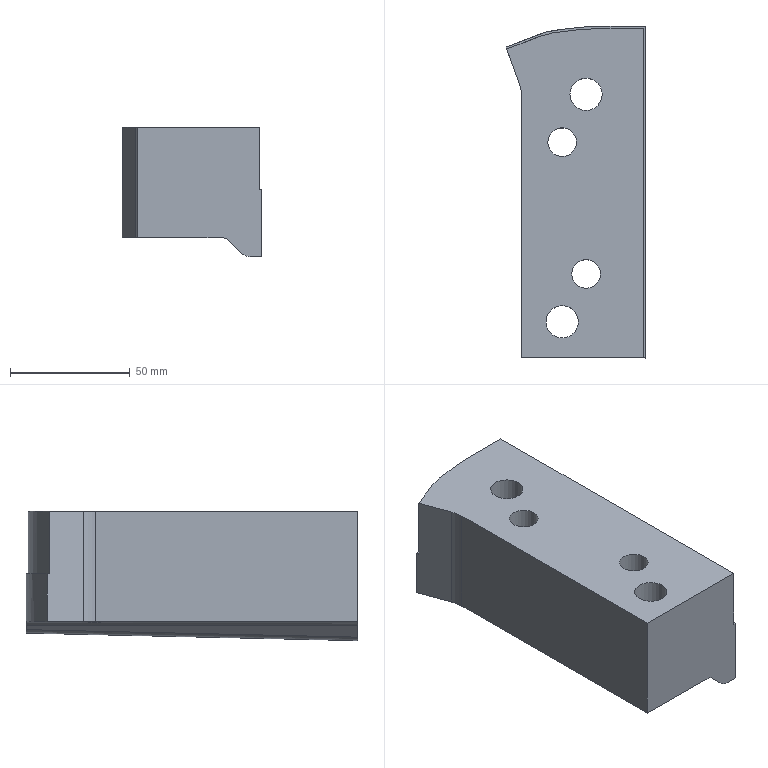Part | NX | features solid 2 | 1 solid | 27 faces | box 58.448 x 138.583 x 54 mm | volume 307683 mm3 | plane 14 | cylinder 11 | spline 2 | commonest cylinder face diameters 10 x2 12 x2 13 x2 13.5 x2 19.5 x2 30 x1
STEP:
#1=CARTESIAN_POINT('',(-128.106,-103.122,40.));
#2=VERTEX_POINT('',#1);
#3=CARTESIAN_POINT('',(-71.,-94.425,40.));
#4=VERTEX_POINT('',#3);
#5=CARTESIAN_POINT('',(-128.106,-103.122,40.));
#6=CARTESIAN_POINT('',(-125.791,-102.343,40.));
#7=CARTESIAN_POINT('',(-121.178,-100.674,40.));
#8=CARTESIAN_POINT('',(-115.494,-98.056,40.));
#9=CARTESIAN_POINT('',(-110.841,-96.645,40.));
#10=CARTESIAN_POINT('',(-107.28,-96.048,40.));
#11=CARTESIAN_POINT('',(-103.692,-95.631,40.));
#12=CARTESIAN_POINT('',(-98.907,-95.073,40.));
#13=CARTESIAN_POINT('',(-92.898,-94.557,40.));
#14=CARTESIAN_POINT('',(-85.612,-94.429,40.));
#15=CARTESIAN_POINT('',(-78.299,-94.474,40.));
#16=CARTESIAN_POINT('',(-73.433,-94.443,40.));
#17=CARTESIAN_POINT('',(-71.,-94.425,40.));
#18=B_SPLINE_CURVE_WITH_KNOTS('',3,(#5,#6,#7,#8,#9,#10,#11,#12,#13,#14,#15,#16,#17),.UNSPECIFIED.,.F.,.F.,(4,1,1,1,1,1,1,1,1,1,4),(0.0007141,0.007935,0.01516,0.01877,0.02238,0.02599,0.0296,0.03682,0.04404,0.05126,0.05848),.UNSPECIFIED.);
#19=EDGE_CURVE('',#2,#4,#18,.T.);
#20=ORIENTED_EDGE('',*,*,#19,.F.);
#21=CARTESIAN_POINT('',(-122.905,-117.413,40.));
#22=VERTEX_POINT('',#21);
#23=CARTESIAN_POINT('',(-206.143,111.282,40.));
#24=DIRECTION('',(0.342,-0.9397,0.));
#25=VECTOR('',#24,1000.);
#26=LINE('',#23,#25);
#27=EDGE_CURVE('',#2,#22,#26,.T.);
#28=ORIENTED_EDGE('',*,*,#27,.T.);
#29=CARTESIAN_POINT('',(-122.,-122.543,40.));
#30=VERTEX_POINT('',#29);
#31=CARTESIAN_POINT('',(-137.,-122.543,40.));
#32=DIRECTION('',(0.,0.,1.));
#33=DIRECTION('',(1.,0.,0.));
#34=AXIS2_PLACEMENT_3D('',#31,#32,#33);
#35=CIRCLE('',#34,15.);
#36=EDGE_CURVE('',#22,#30,#35,.F.);
#37=ORIENTED_EDGE('',*,*,#36,.T.);
#38=CARTESIAN_POINT('',(-122.,-232.,40.));
#39=VERTEX_POINT('',#38);
#40=CARTESIAN_POINT('',(-122.,35.09,40.));
#41=DIRECTION('',(0.,1.,0.));
#42=VECTOR('',#41,1000.);
#43=LINE('',#40,#42);
#44=EDGE_CURVE('',#39,#30,#43,.T.);
#45=ORIENTED_EDGE('',*,*,#44,.F.);
#46=CARTESIAN_POINT('',(-71.,-232.,40.));
#47=VERTEX_POINT('',#46);
#48=CARTESIAN_POINT('',(-415.478,-232.,40.));
#49=DIRECTION('',(1.,0.,0.));
#50=VECTOR('',#49,1000.);
#51=LINE('',#48,#50);
#52=EDGE_CURVE('',#47,#39,#51,.F.);
#53=ORIENTED_EDGE('',*,*,#52,.F.);
#54=CARTESIAN_POINT('',(-71.,35.09,40.));
#55=DIRECTION('',(0.,1.,0.));
#56=VECTOR('',#55,1000.);
#57=LINE('',#54,#56);
#58=EDGE_CURVE('',#47,#4,#57,.T.);
#59=ORIENTED_EDGE('',*,*,#58,.T.);
#60=EDGE_LOOP('',(#20,#28,#37,#45,#53,#59));
#61=FACE_BOUND('',#60,.T.);
#62=CARTESIAN_POINT('',(-89.,-197.,40.));
#63=VERTEX_POINT('',#62);
#64=CARTESIAN_POINT('',(-95.,-197.,40.));
#65=DIRECTION('',(0.,0.,1.));
#66=DIRECTION('',(1.,0.,0.));
#67=AXIS2_PLACEMENT_3D('',#64,#65,#66);
#68=CIRCLE('',#67,6.);
#69=EDGE_CURVE('',#63,#63,#68,.T.);
#70=ORIENTED_EDGE('',*,*,#69,.F.);
#71=EDGE_LOOP('',(#70));
#72=FACE_BOUND('',#71,.T.);
#73=CARTESIAN_POINT('',(-99.,-142.,40.));
#74=VERTEX_POINT('',#73);
#75=CARTESIAN_POINT('',(-105.,-142.,40.));
#76=DIRECTION('',(0.,0.,1.));
#77=DIRECTION('',(1.,0.,0.));
#78=AXIS2_PLACEMENT_3D('',#75,#76,#77);
#79=CIRCLE('',#78,6.);
#80=EDGE_CURVE('',#74,#74,#79,.T.);
#81=ORIENTED_EDGE('',*,*,#80,.F.);
#82=EDGE_LOOP('',(#81));
#83=FACE_BOUND('',#82,.T.);
#84=CARTESIAN_POINT('',(-88.25,-122.,40.));
#85=VERTEX_POINT('',#84);
#86=CARTESIAN_POINT('',(-95.,-122.,40.));
#87=DIRECTION('',(0.,0.,1.));
#88=DIRECTION('',(1.,0.,0.));
#89=AXIS2_PLACEMENT_3D('',#86,#87,#88);
#90=CIRCLE('',#89,6.75);
#91=EDGE_CURVE('',#85,#85,#90,.T.);
#92=ORIENTED_EDGE('',*,*,#91,.F.);
#93=EDGE_LOOP('',(#92));
#94=FACE_BOUND('',#93,.T.);
#95=CARTESIAN_POINT('',(-98.25,-217.,40.));
#96=VERTEX_POINT('',#95);
#97=CARTESIAN_POINT('',(-105.,-217.,40.));
#98=DIRECTION('',(0.,0.,1.));
#99=DIRECTION('',(1.,0.,0.));
#100=AXIS2_PLACEMENT_3D('',#97,#98,#99);
#101=CIRCLE('',#100,6.75);
#102=EDGE_CURVE('',#96,#96,#101,.T.);
#103=ORIENTED_EDGE('',*,*,#102,.F.);
#104=EDGE_LOOP('',(#103));
#105=FACE_BOUND('',#104,.T.);
#106=CARTESIAN_POINT('',(-415.478,35.09,40.));
#107=DIRECTION('',(0.,0.,1.));
#108=DIRECTION('',(1.,0.,0.));
#109=AXIS2_PLACEMENT_3D('',#106,#107,#108);
#110=PLANE('',#109);
#111=ADVANCED_FACE('',(#61,#72,#83,#94,#105),#110,.T.);
#112=CARTESIAN_POINT('',(-70.,-93.417,14.));
#113=VERTEX_POINT('',#112);
#114=CARTESIAN_POINT('',(-70.,-232.,14.));
#115=VERTEX_POINT('',#114);
#116=CARTESIAN_POINT('',(-70.,-99.381,14.));
#117=DIRECTION('',(0.,-1.,0.));
#118=VECTOR('',#117,1000.);
#119=LINE('',#116,#118);
#120=EDGE_CURVE('',#113,#115,#119,.T.);
#121=ORIENTED_EDGE('',*,*,#120,.T.);
#122=CARTESIAN_POINT('',(-70.,-232.,-14.));
#123=VERTEX_POINT('',#122);
#124=CARTESIAN_POINT('',(-70.,-232.,-66.));
#125=DIRECTION('',(0.,0.,1.));
#126=VECTOR('',#125,1000.);
#127=LINE('',#124,#126);
#128=EDGE_CURVE('',#115,#123,#127,.F.);
#129=ORIENTED_EDGE('',*,*,#128,.T.);
#130=CARTESIAN_POINT('',(-70.,-93.417,-10.865));
#131=VERTEX_POINT('',#130);
#132=CARTESIAN_POINT('',(-70.,-231.932,-13.998));
#133=DIRECTION('',(0.,0.9997,0.02262));
#134=VECTOR('',#133,1000.);
#135=LINE('',#132,#134);
#136=EDGE_CURVE('',#123,#131,#135,.T.);
#137=ORIENTED_EDGE('',*,*,#136,.T.);
#138=CARTESIAN_POINT('',(-70.,-93.417,1.5));
#139=DIRECTION('',(0.,0.,-1.));
#140=VECTOR('',#139,1000.);
#141=LINE('',#138,#140);
#142=EDGE_CURVE('',#131,#113,#141,.F.);
#143=ORIENTED_EDGE('',*,*,#142,.T.);
#144=EDGE_LOOP('',(#121,#129,#137,#143));
#145=FACE_BOUND('',#144,.T.);
#146=CARTESIAN_POINT('',(-70.,-99.381,-66.));
#147=DIRECTION('',(-1.,0.,0.));
#148=DIRECTION('',(0.,0.,1.));
#149=AXIS2_PLACEMENT_3D('',#146,#147,#148);
#150=PLANE('',#149);
#151=ADVANCED_FACE('',(#145),#150,.F.);
#152=CARTESIAN_POINT('',(-83.536,-232.,-7.464));
#153=VERTEX_POINT('',#152);
#154=CARTESIAN_POINT('',(-78.467,-232.,-12.533));
#155=VERTEX_POINT('',#154);
#156=CARTESIAN_POINT('',(-42.,-232.,-49.));
#157=DIRECTION('',(0.7071,0.,-0.7071));
#158=VECTOR('',#157,1000.);
#159=LINE('',#156,#158);
#160=EDGE_CURVE('',#153,#155,#159,.T.);
#161=ORIENTED_EDGE('',*,*,#160,.T.);
#162=CARTESIAN_POINT('',(-74.929,-232.,-13.999));
#163=VERTEX_POINT('',#162);
#164=CARTESIAN_POINT('',(-74.931,-232.,-8.998));
#165=DIRECTION('',(0.,-1.,0.));
#166=DIRECTION('',(0.7071,0.,-0.7071));
#167=AXIS2_PLACEMENT_3D('',#164,#165,#166);
#168=ELLIPSE('',#167,5.003,5.);
#169=EDGE_CURVE('',#155,#163,#168,.T.);
#170=ORIENTED_EDGE('',*,*,#169,.T.);
#171=CARTESIAN_POINT('',(-90.001,-232.,-13.996));
#172=DIRECTION('',(1.,0.,-0.0001826));
#173=VECTOR('',#172,1000.);
#174=LINE('',#171,#173);
#175=EDGE_CURVE('',#163,#123,#174,.T.);
#176=ORIENTED_EDGE('',*,*,#175,.T.);
#177=ORIENTED_EDGE('',*,*,#128,.F.);
#178=CARTESIAN_POINT('',(-71.,-232.,14.));
#179=VERTEX_POINT('',#178);
#180=CARTESIAN_POINT('',(-454.349,-232.,14.));
#181=DIRECTION('',(-1.,0.,0.));
#182=VECTOR('',#181,1000.);
#183=LINE('',#180,#182);
#184=EDGE_CURVE('',#179,#115,#183,.F.);
#185=ORIENTED_EDGE('',*,*,#184,.F.);
#186=CARTESIAN_POINT('',(-71.,-232.,14.));
#187=DIRECTION('',(0.,0.,-1.));
#188=VECTOR('',#187,1000.);
#189=LINE('',#186,#188);
#190=EDGE_CURVE('',#179,#47,#189,.F.);
#191=ORIENTED_EDGE('',*,*,#190,.T.);
#192=ORIENTED_EDGE('',*,*,#52,.T.);
#193=CARTESIAN_POINT('',(-122.,-232.,-6.));
#194=VERTEX_POINT('',#193);
#195=CARTESIAN_POINT('',(-122.,-232.,-67.));
#196=DIRECTION('',(0.,0.,1.));
#197=VECTOR('',#196,1000.);
#198=LINE('',#195,#197);
#199=EDGE_CURVE('',#39,#194,#198,.F.);
#200=ORIENTED_EDGE('',*,*,#199,.T.);
#201=CARTESIAN_POINT('',(-87.071,-232.,-6.));
#202=VERTEX_POINT('',#201);
#203=CARTESIAN_POINT('',(-470.381,-232.,-6.));
#204=DIRECTION('',(-1.,0.,0.));
#205=VECTOR('',#204,1000.);
#206=LINE('',#203,#205);
#207=EDGE_CURVE('',#194,#202,#206,.F.);
#208=ORIENTED_EDGE('',*,*,#207,.T.);
#209=CARTESIAN_POINT('',(-87.071,-232.,-11.));
#210=DIRECTION('',(0.,-1.,0.));
#211=DIRECTION('',(0.,0.,-1.));
#212=AXIS2_PLACEMENT_3D('',#209,#210,#211);
#213=CIRCLE('',#212,5.);
#214=EDGE_CURVE('',#202,#153,#213,.F.);
#215=ORIENTED_EDGE('',*,*,#214,.T.);
#216=EDGE_LOOP('',(#161,#170,#176,#177,#185,#191,#192,#200,#208,#215));
#217=FACE_BOUND('',#216,.T.);
#218=CARTESIAN_POINT('',(-70.,-232.,-67.));
#219=DIRECTION('',(0.,-1.,0.));
#220=DIRECTION('',(0.,0.,1.));
#221=AXIS2_PLACEMENT_3D('',#218,#219,#220);
#222=PLANE('',#221);
#223=ADVANCED_FACE('',(#217),#222,.T.);
#224=CARTESIAN_POINT('',(-88.5,-197.,-6.));
#225=VERTEX_POINT('',#224);
#226=CARTESIAN_POINT('',(-95.,-197.,-6.));
#227=DIRECTION('',(0.,0.,1.));
#228=DIRECTION('',(1.,0.,0.));
#229=AXIS2_PLACEMENT_3D('',#226,#227,#228);
#230=CIRCLE('',#229,6.5);
#231=EDGE_CURVE('',#225,#225,#230,.T.);
#232=ORIENTED_EDGE('',*,*,#231,.T.);
#233=EDGE_LOOP('',(#232));
#234=FACE_BOUND('',#233,.T.);
#235=CARTESIAN_POINT('',(-98.5,-142.,-6.));
#236=VERTEX_POINT('',#235);
#237=CARTESIAN_POINT('',(-105.,-142.,-6.));
#238=DIRECTION('',(0.,0.,1.));
#239=DIRECTION('',(1.,0.,0.));
#240=AXIS2_PLACEMENT_3D('',#237,#238,#239);
#241=CIRCLE('',#240,6.5);
#242=EDGE_CURVE('',#236,#236,#241,.T.);
#243=ORIENTED_EDGE('',*,*,#242,.T.);
#244=EDGE_LOOP('',(#243));
#245=FACE_BOUND('',#244,.T.);
#246=CARTESIAN_POINT('',(-128.448,-102.182,-6.));
#247=VERTEX_POINT('',#246);
#248=CARTESIAN_POINT('',(-87.071,-93.469,-6.));
#249=VERTEX_POINT('',#248);
#250=CARTESIAN_POINT('',(-128.448,-102.182,-6.));
#251=CARTESIAN_POINT('',(-126.732,-101.605,-6.));
#252=CARTESIAN_POINT('',(-123.317,-100.412,-6.));
#253=CARTESIAN_POINT('',(-118.327,-98.259,-6.));
#254=CARTESIAN_POINT('',(-113.316,-96.192,-6.));
#255=CARTESIAN_POINT('',(-108.153,-95.109,-6.));
#256=CARTESIAN_POINT('',(-102.907,-94.545,-6.));
#257=CARTESIAN_POINT('',(-97.669,-93.925,-6.));
#258=CARTESIAN_POINT('',(-92.389,-93.579,-6.));
#259=CARTESIAN_POINT('',(-88.846,-93.489,-6.));
#260=CARTESIAN_POINT('',(-87.071,-93.469,-6.));
#261=B_SPLINE_CURVE_WITH_KNOTS('',3,(#250,#251,#252,#253,#254,#255,#256,#257,#258,#259,#260),.UNSPECIFIED.,.F.,.F.,(4,1,1,1,1,1,1,1,4),(-0.008773,-0.003503,0.001767,0.007037,0.01231,0.01758,0.02285,0.02812,0.03339),.UNSPECIFIED.);
#262=EDGE_CURVE('',#247,#249,#261,.T.);
#263=ORIENTED_EDGE('',*,*,#262,.T.);
#264=CARTESIAN_POINT('',(-87.071,-116.326,-6.));
#265=VERTEX_POINT('',#264);
#266=CARTESIAN_POINT('',(-87.071,-222.,-6.));
#267=DIRECTION('',(0.,1.,0.));
#268=VECTOR('',#267,1000.);
#269=LINE('',#266,#268);
#270=EDGE_CURVE('',#249,#265,#269,.F.);
#271=ORIENTED_EDGE('',*,*,#270,.T.);
#272=CARTESIAN_POINT('',(-87.071,-127.674,-6.));
#273=VERTEX_POINT('',#272);
#274=CARTESIAN_POINT('',(-95.,-122.,-6.));
#275=DIRECTION('',(0.,0.,1.));
#276=DIRECTION('',(1.,0.,0.));
#277=AXIS2_PLACEMENT_3D('',#274,#275,#276);
#278=CIRCLE('',#277,9.75);
#279=EDGE_CURVE('',#265,#273,#278,.T.);
#280=ORIENTED_EDGE('',*,*,#279,.T.);
#281=CARTESIAN_POINT('',(-87.071,-222.,-6.));
#282=DIRECTION('',(0.,1.,0.));
#283=VECTOR('',#282,1000.);
#284=LINE('',#281,#283);
#285=EDGE_CURVE('',#273,#202,#284,.F.);
#286=ORIENTED_EDGE('',*,*,#285,.T.);
#287=ORIENTED_EDGE('',*,*,#207,.F.);
#288=CARTESIAN_POINT('',(-122.,-122.543,-6.));
#289=VERTEX_POINT('',#288);
#290=CARTESIAN_POINT('',(-122.,-222.,-6.));
#291=DIRECTION('',(0.,-1.,0.));
#292=VECTOR('',#291,1000.);
#293=LINE('',#290,#292);
#294=EDGE_CURVE('',#289,#194,#293,.T.);
#295=ORIENTED_EDGE('',*,*,#294,.F.);
#296=CARTESIAN_POINT('',(-122.905,-117.413,-6.));
#297=VERTEX_POINT('',#296);
#298=CARTESIAN_POINT('',(-137.,-122.543,-6.));
#299=DIRECTION('',(0.,0.,-1.));
#300=DIRECTION('',(-1.,0.,0.));
#301=AXIS2_PLACEMENT_3D('',#298,#299,#300);
#302=CIRCLE('',#301,15.);
#303=EDGE_CURVE('',#289,#297,#302,.F.);
#304=ORIENTED_EDGE('',*,*,#303,.T.);
#305=CARTESIAN_POINT('',(-129.938,-98.089,-6.));
#306=DIRECTION('',(-0.342,0.9397,0.));
#307=VECTOR('',#306,1000.);
#308=LINE('',#305,#307);
#309=EDGE_CURVE('',#297,#247,#308,.T.);
#310=ORIENTED_EDGE('',*,*,#309,.T.);
#311=EDGE_LOOP('',(#263,#271,#280,#286,#287,#295,#304,#310));
#312=FACE_BOUND('',#311,.T.);
#313=CARTESIAN_POINT('',(-95.25,-217.,-6.));
#314=VERTEX_POINT('',#313);
#315=CARTESIAN_POINT('',(-105.,-217.,-6.));
#316=DIRECTION('',(0.,0.,1.));
#317=DIRECTION('',(1.,0.,0.));
#318=AXIS2_PLACEMENT_3D('',#315,#316,#317);
#319=CIRCLE('',#318,9.75);
#320=EDGE_CURVE('',#314,#314,#319,.T.);
#321=ORIENTED_EDGE('',*,*,#320,.T.);
#322=EDGE_LOOP('',(#321));
#323=FACE_BOUND('',#322,.T.);
#324=CARTESIAN_POINT('',(-470.381,-222.,-6.));
#325=DIRECTION('',(0.,0.,-1.));
#326=DIRECTION('',(-1.,0.,0.));
#327=AXIS2_PLACEMENT_3D('',#324,#325,#326);
#328=PLANE('',#327);
#329=ADVANCED_FACE('',(#234,#245,#312,#323),#328,.T.);
#330=CARTESIAN_POINT('',(-78.064,-93.458,-10.865));
#331=VERTEX_POINT('',#330);
#332=CARTESIAN_POINT('',(-78.064,-93.458,-10.865));
#333=CARTESIAN_POINT('',(-75.376,-93.455,-10.865));
#334=CARTESIAN_POINT('',(-72.688,-93.438,-10.865));
#335=CARTESIAN_POINT('',(-70.,-93.417,-10.865));
#336=B_SPLINE_CURVE_WITH_KNOTS('',3,(#332,#333,#334,#335),.UNSPECIFIED.,.F.,.F.,(4,4),(0.002072,0.01014),.UNSPECIFIED.);
#337=EDGE_CURVE('',#331,#131,#336,.T.);
#338=ORIENTED_EDGE('',*,*,#337,.F.);
#339=CARTESIAN_POINT('',(-81.601,-93.455,-9.399));
#340=VERTEX_POINT('',#339);
#341=CARTESIAN_POINT('',(-78.064,-93.458,-10.865));
#342=CARTESIAN_POINT('',(-79.385,-93.46,-10.864));
#343=CARTESIAN_POINT('',(-80.667,-93.457,-10.333));
#344=CARTESIAN_POINT('',(-81.601,-93.455,-9.399));
#345=B_SPLINE_CURVE_WITH_KNOTS('',3,(#341,#342,#343,#344),.UNSPECIFIED.,.F.,.F.,(4,4),(0.,0.003906),.UNSPECIFIED.);
#346=EDGE_CURVE('',#331,#340,#345,.T.);
#347=ORIENTED_EDGE('',*,*,#346,.T.);
#348=CARTESIAN_POINT('',(-83.536,-93.453,-7.464));
#349=VERTEX_POINT('',#348);
#350=CARTESIAN_POINT('',(-81.601,-93.455,-9.399));
#351=CARTESIAN_POINT('',(-82.246,-93.454,-8.754));
#352=CARTESIAN_POINT('',(-82.891,-93.453,-8.109));
#353=CARTESIAN_POINT('',(-83.536,-93.453,-7.464));
#354=B_SPLINE_CURVE_WITH_KNOTS('',3,(#350,#351,#352,#353),.UNSPECIFIED.,.F.,.F.,(4,4),(0.002072,0.004808),.UNSPECIFIED.);
#355=EDGE_CURVE('',#340,#349,#354,.T.);
#356=ORIENTED_EDGE('',*,*,#355,.T.);
#357=CARTESIAN_POINT('',(-83.536,-93.453,-7.464));
#358=CARTESIAN_POINT('',(-84.469,-93.453,-6.531));
#359=CARTESIAN_POINT('',(-85.751,-93.455,-6.));
#360=CARTESIAN_POINT('',(-87.071,-93.469,-6.));
#361=B_SPLINE_CURVE_WITH_KNOTS('',3,(#357,#358,#359,#360),.UNSPECIFIED.,.F.,.F.,(4,4),(0.,0.003904),.UNSPECIFIED.);
#362=EDGE_CURVE('',#349,#249,#361,.T.);
#363=ORIENTED_EDGE('',*,*,#362,.T.);
#364=ORIENTED_EDGE('',*,*,#262,.F.);
#365=CARTESIAN_POINT('',(-128.448,-102.182,14.));
#366=VERTEX_POINT('',#365);
#367=CARTESIAN_POINT('',(-128.448,-102.182,15.35));
#368=DIRECTION('',(0.,0.,-1.));
#369=VECTOR('',#368,1000.);
#370=LINE('',#367,#369);
#371=EDGE_CURVE('',#247,#366,#370,.F.);
#372=ORIENTED_EDGE('',*,*,#371,.T.);
#373=CARTESIAN_POINT('',(-71.,-93.425,14.));
#374=VERTEX_POINT('',#373);
#375=CARTESIAN_POINT('',(-190.231,-121.49,14.));
#376=CARTESIAN_POINT('',(-188.654,-121.152,14.));
#377=CARTESIAN_POINT('',(-185.47,-120.627,14.));
#378=CARTESIAN_POINT('',(-180.656,-120.141,14.));
#379=CARTESIAN_POINT('',(-175.882,-119.326,14.));
#380=CARTESIAN_POINT('',(-169.679,-117.528,14.));
#381=CARTESIAN_POINT('',(-162.185,-114.539,14.));
#382=CARTESIAN_POINT('',(-153.086,-111.254,14.));
#383=CARTESIAN_POINT('',(-144.031,-107.845,14.));
#384=CARTESIAN_POINT('',(-136.465,-105.061,14.));
#385=CARTESIAN_POINT('',(-130.418,-102.814,14.));
#386=CARTESIAN_POINT('',(-125.812,-101.329,14.));
#387=CARTESIAN_POINT('',(-121.306,-99.566,14.));
#388=CARTESIAN_POINT('',(-116.876,-97.626,14.));
#389=CARTESIAN_POINT('',(-112.335,-95.923,14.));
#390=CARTESIAN_POINT('',(-107.564,-95.05,14.));
#391=CARTESIAN_POINT('',(-102.756,-94.525,14.));
#392=CARTESIAN_POINT('',(-96.349,-93.771,14.));
#393=CARTESIAN_POINT('',(-89.902,-93.468,14.));
#394=CARTESIAN_POINT('',(-83.452,-93.448,14.));
#395=CARTESIAN_POINT('',(-77.002,-93.469,14.));
#396=CARTESIAN_POINT('',(-68.939,-93.411,14.));
#397=CARTESIAN_POINT('',(-56.04,-93.3,14.));
#398=CARTESIAN_POINT('',(-33.465,-93.184,14.));
#399=CARTESIAN_POINT('',(-7.666,-93.074,14.));
#400=CARTESIAN_POINT('',(14.907,-92.653,14.));
#401=CARTESIAN_POINT('',(27.794,-92.068,14.));
#402=CARTESIAN_POINT('',(40.668,-91.245,14.));
#403=CARTESIAN_POINT('',(51.917,-90.291,14.));
#404=CARTESIAN_POINT('',(61.528,-89.174,14.));
#405=CARTESIAN_POINT('',(67.939,-88.466,14.));
#406=CARTESIAN_POINT('',(79.125,-86.95,14.));
#407=CARTESIAN_POINT('',(95.161,-85.253,14.));
#408=CARTESIAN_POINT('',(114.404,-83.21,14.));
#409=CARTESIAN_POINT('',(133.568,-80.524,14.));
#410=CARTESIAN_POINT('',(152.734,-77.861,14.));
#411=CARTESIAN_POINT('',(171.916,-75.326,14.));
#412=CARTESIAN_POINT('',(191.055,-72.413,14.));
#413=CARTESIAN_POINT('',(207.17,-71.468,14.));
#414=CARTESIAN_POINT('',(219.951,-69.697,14.));
#415=CARTESIAN_POINT('',(232.724,-67.899,14.));
#416=CARTESIAN_POINT('',(248.708,-65.766,14.));
#417=CARTESIAN_POINT('',(267.87,-63.074,14.));
#418=CARTESIAN_POINT('',(287.038,-60.44,14.));
#419=CARTESIAN_POINT('',(301.448,-58.682,14.));
#420=CARTESIAN_POINT('',(310.976,-56.987,14.));
#421=CARTESIAN_POINT('',(314.916,-56.135,14.));
#422=CARTESIAN_POINT('',(318.052,-55.382,14.));
#423=CARTESIAN_POINT('',(320.39,-54.76,14.));
#424=CARTESIAN_POINT('',(322.686,-53.981,14.));
#425=CARTESIAN_POINT('',(325.595,-52.578,14.));
#426=CARTESIAN_POINT('',(328.769,-50.098,14.));
#427=CARTESIAN_POINT('',(332.247,-46.69,14.));
#428=CARTESIAN_POINT('',(335.795,-43.406,14.));
#429=CARTESIAN_POINT('',(343.661,-37.758,14.));
#430=CARTESIAN_POINT('',(355.164,-28.914,14.));
#431=CARTESIAN_POINT('',(370.422,-17.018,14.));
#432=CARTESIAN_POINT('',(383.264,-7.249,14.));
#433=CARTESIAN_POINT('',(392.416,-0.6713,14.));
#434=CARTESIAN_POINT('',(396.953,2.733,14.));
#435=CARTESIAN_POINT('',(398.886,5.372,14.));
#436=CARTESIAN_POINT('',(399.725,7.654,14.));
#437=CARTESIAN_POINT('',(399.76,10.078,14.));
#438=CARTESIAN_POINT('',(399.483,13.317,14.));
#439=CARTESIAN_POINT('',(399.712,17.34,14.));
#440=CARTESIAN_POINT('',(399.612,22.179,14.));
#441=CARTESIAN_POINT('',(399.633,31.854,14.));
#442=CARTESIAN_POINT('',(399.593,46.366,14.));
#443=CARTESIAN_POINT('',(399.637,62.491,14.));
#444=CARTESIAN_POINT('',(399.588,73.779,14.));
#445=CARTESIAN_POINT('',(399.652,79.422,14.));
#446=CARTESIAN_POINT('',(399.59,82.647,14.));
#447=CARTESIAN_POINT('',(399.564,85.065,14.));
#448=CARTESIAN_POINT('',(399.725,87.486,14.));
#449=CARTESIAN_POINT('',(399.756,89.902,14.));
#450=CARTESIAN_POINT('',(399.247,92.301,14.));
#451=CARTESIAN_POINT('',(397.362,95.008,14.));
#452=CARTESIAN_POINT('',(393.635,96.774,14.));
#453=CARTESIAN_POINT('',(389.279,98.826,14.));
#454=CARTESIAN_POINT('',(384.732,100.498,14.));
#455=CARTESIAN_POINT('',(378.765,102.95,14.));
#456=CARTESIAN_POINT('',(362.589,110.229,14.));
#457=CARTESIAN_POINT('',(344.928,118.135,14.));
#458=CARTESIAN_POINT('',(327.281,126.072,14.));
#459=CARTESIAN_POINT('',(319.932,129.381,14.));
#460=CARTESIAN_POINT('',(314.075,132.102,14.));
#461=CARTESIAN_POINT('',(309.387,133.376,14.));
#462=CARTESIAN_POINT('',(304.547,133.785,14.));
#463=CARTESIAN_POINT('',(299.716,133.401,14.));
#464=CARTESIAN_POINT('',(294.929,132.704,14.));
#465=CARTESIAN_POINT('',(288.543,131.8,14.));
#466=CARTESIAN_POINT('',(277.364,130.241,14.));
#467=CARTESIAN_POINT('',(242.2,125.552,14.));
#468=CARTESIAN_POINT('',(184.637,118.048,14.));
#469=CARTESIAN_POINT('',(120.701,109.541,14.));
#470=CARTESIAN_POINT('',(69.531,102.902,14.));
#471=CARTESIAN_POINT('',(40.777,98.94,14.));
#472=CARTESIAN_POINT('',(21.566,96.615,14.));
#473=CARTESIAN_POINT('',(8.743,95.212,14.));
#474=CARTESIAN_POINT('',(-7.301,93.575,14.));
#475=CARTESIAN_POINT('',(-26.625,92.505,14.));
#476=CARTESIAN_POINT('',(-45.971,92.017,14.));
#477=CARTESIAN_POINT('',(-62.09,91.675,14.));
#478=CARTESIAN_POINT('',(-74.987,91.256,14.));
#479=CARTESIAN_POINT('',(-84.664,91.165,14.));
#480=CARTESIAN_POINT('',(-94.319,91.781,14.));
#481=CARTESIAN_POINT('',(-103.929,92.966,14.));
#482=CARTESIAN_POINT('',(-113.495,94.403,14.));
#483=CARTESIAN_POINT('',(-119.856,95.492,14.));
#484=CARTESIAN_POINT('',(-122.997,96.222,14.));
#485=B_SPLINE_CURVE_WITH_KNOTS('',3,(#375,#376,#377,#378,#379,#380,#381,#382,#383,#384,#385,#386,#387,#388,#389,#390,#391,#392,#393,#394,#395,#396,#397,#398,#399,#400,#401,#402,#403,#404,#405,#406,#407,#408,#409,#410,#411,#412,#413,#414,#415,#416,#417,#418,#419,#420,#421,#422,#423,#424,#425,#426,#427,#428,#429,#430,#431,#432,#433,#434,#435,#436,#437,#438,#439,#440,#441,#442,#443,#444,#445,#446,#447,#448,#449,#450,#451,#452,#453,#454,#455,#456,#457,#458,#459,#460,#461,#462,#463,#464,#465,#466,#467,#468,#469,#470,#471,#472,#473,#474,#475,#476,#477,#478,#479,#480,#481,#482,#483,#484),.UNSPECIFIED.,.F.,.F.,(4,1,1,1,1,1,1,1,1,1,1,1,1,1,1,1,1,1,1,1,1,1,1,1,1,1,1,1,1,1,1,1,1,1,1,1,1,1,1,1,1,1,1,1,1,1,1,1,1,1,1,1,1,1,1,1,1,1,1,1,1,1,1,1,1,1,1,1,1,1,1,1,1,1,1,1,1,1,1,1,1,1,1,1,1,1,1,1,1,1,1,1,1,1,1,1,1,1,1,1,1,1,1,1,1,1,1,4),(0.4704,0.4724,0.4745,0.4766,0.4786,0.4828,0.4869,0.491,0.4952,0.4972,0.4993,0.5014,0.5035,0.5055,0.5076,0.5097,0.5117,0.5159,0.5179,0.52,0.5241,0.5283,0.5366,0.5531,0.5614,0.5655,0.5697,0.5779,0.58,0.5821,0.5862,0.5945,0.6028,0.611,0.6193,0.6276,0.6359,0.6441,0.6483,0.6524,0.6607,0.669,0.6772,0.6855,0.6876,0.6897,0.6907,0.6917,0.6928,0.6938,0.6959,0.6979,0.7,0.7021,0.7103,0.7186,0.7269,0.731,0.7331,0.7341,0.7352,0.7362,0.7372,0.7393,0.7414,0.7435,0.7517,0.76,0.7641,0.7662,0.7672,0.7683,0.7693,0.7703,0.7714,0.7724,0.7745,0.7766,0.7786,0.7807,0.7848,0.8014,0.8055,0.8097,0.8117,0.8138,0.8159,0.8179,0.82,0.8221,0.8262,0.8345,0.8676,0.9007,0.9172,0.9338,0.9379,0.9421,0.9503,0.9586,0.9669,0.9752,0.9793,0.9834,0.9876,0.9917,0.9959,1.),.UNSPECIFIED.);
#486=EDGE_CURVE('',#374,#366,#485,.F.);
#487=ORIENTED_EDGE('',*,*,#486,.F.);
#488=CARTESIAN_POINT('',(-70.,-93.417,14.));
#489=CARTESIAN_POINT('',(-70.333,-93.42,14.));
#490=CARTESIAN_POINT('',(-70.667,-93.422,14.));
#491=CARTESIAN_POINT('',(-71.,-93.425,14.));
#492=B_SPLINE_CURVE_WITH_KNOTS('',3,(#488,#489,#490,#491),.UNSPECIFIED.,.F.,.F.,(4,4),(0.,0.0009947),.UNSPECIFIED.);
#493=EDGE_CURVE('',#113,#374,#492,.T.);
#494=ORIENTED_EDGE('',*,*,#493,.F.);
#495=ORIENTED_EDGE('',*,*,#142,.F.);
#496=EDGE_LOOP('',(#338,#347,#356,#363,#364,#372,#487,#494,#495));
#497=FACE_BOUND('',#496,.T.);
#498=CARTESIAN_POINT('',(-128.448,-102.182,14.));
#499=CARTESIAN_POINT('',(-128.448,-102.182,-11.014));
#500=CARTESIAN_POINT('',(-126.088,-101.388,14.));
#501=CARTESIAN_POINT('',(-126.088,-101.388,-11.014));
#502=CARTESIAN_POINT('',(-121.41,-99.687,14.));
#503=CARTESIAN_POINT('',(-121.41,-99.687,-11.014));
#504=CARTESIAN_POINT('',(-115.74,-97.072,14.));
#505=CARTESIAN_POINT('',(-115.74,-97.072,-11.014));
#506=CARTESIAN_POINT('',(-110.967,-95.647,14.));
#507=CARTESIAN_POINT('',(-110.967,-95.647,-11.014));
#508=CARTESIAN_POINT('',(-107.273,-95.036,14.));
#509=CARTESIAN_POINT('',(-107.273,-95.036,-11.014));
#510=CARTESIAN_POINT('',(-103.564,-94.612,14.));
#511=CARTESIAN_POINT('',(-103.564,-94.612,-11.014));
#512=CARTESIAN_POINT('',(-98.617,-94.031,14.));
#513=CARTESIAN_POINT('',(-98.617,-94.031,-11.014));
#514=CARTESIAN_POINT('',(-92.411,-93.532,14.));
#515=CARTESIAN_POINT('',(-92.411,-93.532,-11.014));
#516=CARTESIAN_POINT('',(-84.939,-93.431,14.));
#517=CARTESIAN_POINT('',(-84.939,-93.431,-11.014));
#518=CARTESIAN_POINT('',(-77.47,-93.474,14.));
#519=CARTESIAN_POINT('',(-77.47,-93.474,-11.014));
#520=CARTESIAN_POINT('',(-72.49,-93.436,14.));
#521=CARTESIAN_POINT('',(-72.49,-93.436,-11.014));
#522=CARTESIAN_POINT('',(-70.,-93.417,14.));
#523=CARTESIAN_POINT('',(-70.,-93.417,-11.014));
#524=B_SPLINE_SURFACE_WITH_KNOTS('',3,1,((#498,#499),(#500,#501),(#502,#503),(#504,#505),(#506,#507),(#508,#509),(#510,#511),(#512,#513),(#514,#515),(#516,#517),(#518,#519),(#520,#521),(#522,#523)),.SURF_OF_LINEAR_EXTRUSION.,.F.,.F.,.F.,(4,1,1,1,1,1,1,1,1,1,4),(2,2),(0.4981,0.5013,0.5045,0.5061,0.5077,0.5093,0.5109,0.5141,0.5173,0.5205,0.5237),(0.,1.),.UNSPECIFIED.);
#525=ADVANCED_FACE('',(#497),#524,.T.);
#526=ORIENTED_EDGE('',*,*,#44,.T.);
#527=CARTESIAN_POINT('',(-122.,-122.543,23.));
#528=DIRECTION('',(0.,0.,-1.));
#529=VECTOR('',#528,1000.);
#530=LINE('',#527,#529);
#531=EDGE_CURVE('',#30,#289,#530,.T.);
#532=ORIENTED_EDGE('',*,*,#531,.T.);
#533=ORIENTED_EDGE('',*,*,#294,.T.);
#534=ORIENTED_EDGE('',*,*,#199,.F.);
#535=EDGE_LOOP('',(#526,#532,#533,#534));
#536=FACE_BOUND('',#535,.T.);
#537=CARTESIAN_POINT('',(-122.,-169.69,23.));
#538=DIRECTION('',(1.,0.,0.));
#539=DIRECTION('',(0.,0.,-1.));
#540=AXIS2_PLACEMENT_3D('',#537,#538,#539);
#541=PLANE('',#540);
#542=ADVANCED_FACE('',(#536),#541,.F.);
#543=ORIENTED_EDGE('',*,*,#184,.T.);
#544=ORIENTED_EDGE('',*,*,#120,.F.);
#545=ORIENTED_EDGE('',*,*,#493,.T.);
#546=ORIENTED_EDGE('',*,*,#486,.T.);
#547=CARTESIAN_POINT('',(-128.106,-103.122,14.));
#548=VERTEX_POINT('',#547);
#549=CARTESIAN_POINT('',(-129.506,-99.275,14.));
#550=DIRECTION('',(0.342,-0.9397,0.));
#551=VECTOR('',#550,1000.);
#552=LINE('',#549,#551);
#553=EDGE_CURVE('',#366,#548,#552,.T.);
#554=ORIENTED_EDGE('',*,*,#553,.T.);
#555=CARTESIAN_POINT('',(-71.,-94.425,14.));
#556=VERTEX_POINT('',#555);
#557=CARTESIAN_POINT('',(-128.106,-103.122,14.));
#558=CARTESIAN_POINT('',(-125.786,-102.341,14.));
#559=CARTESIAN_POINT('',(-121.105,-100.639,14.));
#560=CARTESIAN_POINT('',(-115.535,-98.084,14.));
#561=CARTESIAN_POINT('',(-111.035,-96.692,14.));
#562=CARTESIAN_POINT('',(-107.497,-96.076,14.));
#563=CARTESIAN_POINT('',(-103.881,-95.651,14.));
#564=CARTESIAN_POINT('',(-99.007,-95.085,14.));
#565=CARTESIAN_POINT('',(-92.989,-94.561,14.));
#566=CARTESIAN_POINT('',(-85.691,-94.429,14.));
#567=CARTESIAN_POINT('',(-78.349,-94.474,14.));
#568=CARTESIAN_POINT('',(-73.448,-94.443,14.));
#569=CARTESIAN_POINT('',(-71.,-94.425,14.));
#570=B_SPLINE_CURVE_WITH_KNOTS('',3,(#557,#558,#559,#560,#561,#562,#563,#564,#565,#566,#567,#568,#569),.UNSPECIFIED.,.F.,.F.,(4,1,1,1,1,1,1,1,1,1,4),(0.4981,0.5013,0.5044,0.506,0.5076,0.5091,0.5107,0.5138,0.517,0.5201,0.5233),.UNSPECIFIED.);
#571=EDGE_CURVE('',#548,#556,#570,.T.);
#572=ORIENTED_EDGE('',*,*,#571,.T.);
#573=CARTESIAN_POINT('',(-71.,-240.,14.));
#574=DIRECTION('',(0.,1.,0.));
#575=VECTOR('',#574,1000.);
#576=LINE('',#573,#575);
#577=EDGE_CURVE('',#179,#556,#576,.T.);
#578=ORIENTED_EDGE('',*,*,#577,.F.);
#579=EDGE_LOOP('',(#543,#544,#545,#546,#554,#572,#578));
#580=FACE_BOUND('',#579,.T.);
#581=CARTESIAN_POINT('',(-454.349,119.974,14.));
#582=DIRECTION('',(0.,0.,-1.));
#583=DIRECTION('',(-1.,0.,0.));
#584=AXIS2_PLACEMENT_3D('',#581,#582,#583);
#585=PLANE('',#584);
#586=ADVANCED_FACE('',(#580),#585,.F.);
#587=CARTESIAN_POINT('',(-71.,-94.425,57.));
#588=DIRECTION('',(0.,0.,1.));
#589=VECTOR('',#588,1000.);
#590=LINE('',#587,#589);
#591=EDGE_CURVE('',#4,#556,#590,.F.);
#592=ORIENTED_EDGE('',*,*,#591,.F.);
#593=ORIENTED_EDGE('',*,*,#58,.F.);
#594=ORIENTED_EDGE('',*,*,#190,.F.);
#595=ORIENTED_EDGE('',*,*,#577,.T.);
#596=EDGE_LOOP('',(#592,#593,#594,#595));
#597=FACE_BOUND('',#596,.T.);
#598=CARTESIAN_POINT('',(-71.,-240.,14.));
#599=DIRECTION('',(1.,0.,0.));
#600=DIRECTION('',(0.,0.,-1.));
#601=AXIS2_PLACEMENT_3D('',#598,#599,#600);
#602=PLANE('',#601);
#603=ADVANCED_FACE('',(#597),#602,.T.);
#604=ORIENTED_EDGE('',*,*,#355,.F.);
#605=CARTESIAN_POINT('',(-78.468,-231.931,-12.532));
#606=DIRECTION('',(-0.02261,0.9995,0.02261));
#607=VECTOR('',#606,1000.);
#608=LINE('',#605,#607);
#609=EDGE_CURVE('',#340,#155,#608,.F.);
#610=ORIENTED_EDGE('',*,*,#609,.T.);
#611=ORIENTED_EDGE('',*,*,#160,.F.);
#612=CARTESIAN_POINT('',(-83.536,-232.,-7.464));
#613=DIRECTION('',(0.,-1.,0.));
#614=VECTOR('',#613,1000.);
#615=LINE('',#612,#614);
#616=EDGE_CURVE('',#153,#349,#615,.F.);
#617=ORIENTED_EDGE('',*,*,#616,.T.);
#618=EDGE_LOOP('',(#604,#610,#611,#617));
#619=FACE_BOUND('',#618,.T.);
#620=CARTESIAN_POINT('',(-80.,-232.,-11.));
#621=DIRECTION('',(-0.7071,0.,-0.7071));
#622=DIRECTION('',(-0.7071,0.,0.7071));
#623=AXIS2_PLACEMENT_3D('',#620,#621,#622);
#624=PLANE('',#623);
#625=ADVANCED_FACE('',(#619),#624,.T.);
#626=ORIENTED_EDGE('',*,*,#102,.T.);
#627=EDGE_LOOP('',(#626));
#628=FACE_BOUND('',#627,.T.);
#629=CARTESIAN_POINT('',(-98.25,-217.,9.));
#630=VERTEX_POINT('',#629);
#631=CARTESIAN_POINT('',(-105.,-217.,9.));
#632=DIRECTION('',(0.,0.,1.));
#633=DIRECTION('',(1.,0.,0.));
#634=AXIS2_PLACEMENT_3D('',#631,#632,#633);
#635=CIRCLE('',#634,6.75);
#636=EDGE_CURVE('',#630,#630,#635,.T.);
#637=ORIENTED_EDGE('',*,*,#636,.F.);
#638=EDGE_LOOP('',(#637));
#639=FACE_BOUND('',#638,.T.);
#640=CARTESIAN_POINT('',(-105.,-217.,94.));
#641=DIRECTION('',(0.,0.,1.));
#642=DIRECTION('',(1.,0.,0.));
#643=AXIS2_PLACEMENT_3D('',#640,#641,#642);
#644=CYLINDRICAL_SURFACE('',#643,6.75);
#645=ADVANCED_FACE('',(#628,#639),#644,.F.);
#646=ORIENTED_EDGE('',*,*,#636,.T.);
#647=EDGE_LOOP('',(#646));
#648=FACE_BOUND('',#647,.T.);
#649=CARTESIAN_POINT('',(-95.25,-217.,9.));
#650=VERTEX_POINT('',#649);
#651=CARTESIAN_POINT('',(-105.,-217.,9.));
#652=DIRECTION('',(0.,0.,1.));
#653=DIRECTION('',(1.,0.,0.));
#654=AXIS2_PLACEMENT_3D('',#651,#652,#653);
#655=CIRCLE('',#654,9.75);
#656=EDGE_CURVE('',#650,#650,#655,.T.);
#657=ORIENTED_EDGE('',*,*,#656,.F.);
#658=EDGE_LOOP('',(#657));
#659=FACE_BOUND('',#658,.T.);
#660=CARTESIAN_POINT('',(-105.,-217.,9.));
#661=DIRECTION('',(0.,0.,1.));
#662=DIRECTION('',(1.,0.,0.));
#663=AXIS2_PLACEMENT_3D('',#660,#661,#662);
#664=PLANE('',#663);
#665=ADVANCED_FACE('',(#648,#659),#664,.F.);
#666=ORIENTED_EDGE('',*,*,#656,.T.);
#667=EDGE_LOOP('',(#666));
#668=FACE_BOUND('',#667,.T.);
#669=ORIENTED_EDGE('',*,*,#320,.F.);
#670=EDGE_LOOP('',(#669));
#671=FACE_BOUND('',#670,.T.);
#672=CARTESIAN_POINT('',(-105.,-217.,-6.));
#673=DIRECTION('',(0.,0.,1.));
#674=DIRECTION('',(1.,0.,0.));
#675=AXIS2_PLACEMENT_3D('',#672,#673,#674);
#676=CYLINDRICAL_SURFACE('',#675,9.75);
#677=ADVANCED_FACE('',(#668,#671),#676,.F.);
#678=ORIENTED_EDGE('',*,*,#91,.T.);
#679=EDGE_LOOP('',(#678));
#680=FACE_BOUND('',#679,.T.);
#681=CARTESIAN_POINT('',(-88.25,-122.,9.));
#682=VERTEX_POINT('',#681);
#683=CARTESIAN_POINT('',(-95.,-122.,9.));
#684=DIRECTION('',(0.,0.,1.));
#685=DIRECTION('',(1.,0.,0.));
#686=AXIS2_PLACEMENT_3D('',#683,#684,#685);
#687=CIRCLE('',#686,6.75);
#688=EDGE_CURVE('',#682,#682,#687,.T.);
#689=ORIENTED_EDGE('',*,*,#688,.F.);
#690=EDGE_LOOP('',(#689));
#691=FACE_BOUND('',#690,.T.);
#692=CARTESIAN_POINT('',(-95.,-122.,94.));
#693=DIRECTION('',(0.,0.,1.));
#694=DIRECTION('',(1.,0.,0.));
#695=AXIS2_PLACEMENT_3D('',#692,#693,#694);
#696=CYLINDRICAL_SURFACE('',#695,6.75);
#697=ADVANCED_FACE('',(#680,#691),#696,.F.);
#698=ORIENTED_EDGE('',*,*,#688,.T.);
#699=EDGE_LOOP('',(#698));
#700=FACE_BOUND('',#699,.T.);
#701=CARTESIAN_POINT('',(-85.25,-122.,9.));
#702=VERTEX_POINT('',#701);
#703=CARTESIAN_POINT('',(-95.,-122.,9.));
#704=DIRECTION('',(0.,0.,1.));
#705=DIRECTION('',(1.,0.,0.));
#706=AXIS2_PLACEMENT_3D('',#703,#704,#705);
#707=CIRCLE('',#706,9.75);
#708=EDGE_CURVE('',#702,#702,#707,.T.);
#709=ORIENTED_EDGE('',*,*,#708,.F.);
#710=EDGE_LOOP('',(#709));
#711=FACE_BOUND('',#710,.T.);
#712=CARTESIAN_POINT('',(-95.,-112.,9.));
#713=DIRECTION('',(0.,0.,1.));
#714=DIRECTION('',(1.,0.,0.));
#715=AXIS2_PLACEMENT_3D('',#712,#713,#714);
#716=PLANE('',#715);
#717=ADVANCED_FACE('',(#700,#711),#716,.F.);
#718=ORIENTED_EDGE('',*,*,#708,.T.);
#719=EDGE_LOOP('',(#718));
#720=FACE_BOUND('',#719,.T.);
#721=ORIENTED_EDGE('',*,*,#279,.F.);
#722=CARTESIAN_POINT('',(-87.071,-116.326,-6.));
#723=CARTESIAN_POINT('',(-85.887,-117.981,-6.));
#724=CARTESIAN_POINT('',(-84.613,-122.012,-6.687));
#725=CARTESIAN_POINT('',(-85.888,-126.02,-6.));
#726=CARTESIAN_POINT('',(-87.071,-127.674,-6.));
#727=B_SPLINE_CURVE_WITH_KNOTS('',3,(#722,#723,#724,#725,#726),.UNSPECIFIED.,.F.,.F.,(4,1,4),(0.002361,0.008399,0.01444),.UNSPECIFIED.);
#728=EDGE_CURVE('',#273,#265,#727,.F.);
#729=ORIENTED_EDGE('',*,*,#728,.F.);
#730=EDGE_LOOP('',(#721,#729));
#731=FACE_BOUND('',#730,.T.);
#732=CARTESIAN_POINT('',(-95.,-122.,-6.));
#733=DIRECTION('',(0.,0.,1.));
#734=DIRECTION('',(1.,0.,0.));
#735=AXIS2_PLACEMENT_3D('',#732,#733,#734);
#736=CYLINDRICAL_SURFACE('',#735,9.75);
#737=ADVANCED_FACE('',(#720,#731),#736,.F.);
#738=ORIENTED_EDGE('',*,*,#80,.T.);
#739=EDGE_LOOP('',(#738));
#740=FACE_BOUND('',#739,.T.);
#741=CARTESIAN_POINT('',(-99.,-142.,14.));
#742=VERTEX_POINT('',#741);
#743=CARTESIAN_POINT('',(-105.,-142.,14.));
#744=DIRECTION('',(0.,0.,1.));
#745=DIRECTION('',(1.,0.,0.));
#746=AXIS2_PLACEMENT_3D('',#743,#744,#745);
#747=CIRCLE('',#746,6.);
#748=EDGE_CURVE('',#742,#742,#747,.T.);
#749=ORIENTED_EDGE('',*,*,#748,.F.);
#750=EDGE_LOOP('',(#749));
#751=FACE_BOUND('',#750,.T.);
#752=CARTESIAN_POINT('',(-105.,-142.,94.));
#753=DIRECTION('',(0.,0.,1.));
#754=DIRECTION('',(1.,0.,0.));
#755=AXIS2_PLACEMENT_3D('',#752,#753,#754);
#756=CYLINDRICAL_SURFACE('',#755,6.);
#757=ADVANCED_FACE('',(#740,#751),#756,.F.);
#758=ORIENTED_EDGE('',*,*,#748,.T.);
#759=EDGE_LOOP('',(#758));
#760=FACE_BOUND('',#759,.T.);
#761=CARTESIAN_POINT('',(-98.5,-142.,14.));
#762=VERTEX_POINT('',#761);
#763=CARTESIAN_POINT('',(-105.,-142.,14.));
#764=DIRECTION('',(0.,0.,1.));
#765=DIRECTION('',(1.,0.,0.));
#766=AXIS2_PLACEMENT_3D('',#763,#764,#765);
#767=CIRCLE('',#766,6.5);
#768=EDGE_CURVE('',#762,#762,#767,.T.);
#769=ORIENTED_EDGE('',*,*,#768,.F.);
#770=EDGE_LOOP('',(#769));
#771=FACE_BOUND('',#770,.T.);
#772=CARTESIAN_POINT('',(-105.,-142.,14.));
#773=DIRECTION('',(0.,0.,1.));
#774=DIRECTION('',(1.,0.,0.));
#775=AXIS2_PLACEMENT_3D('',#772,#773,#774);
#776=PLANE('',#775);
#777=ADVANCED_FACE('',(#760,#771),#776,.F.);
#778=ORIENTED_EDGE('',*,*,#768,.T.);
#779=EDGE_LOOP('',(#778));
#780=FACE_BOUND('',#779,.T.);
#781=ORIENTED_EDGE('',*,*,#242,.F.);
#782=EDGE_LOOP('',(#781));
#783=FACE_BOUND('',#782,.T.);
#784=CARTESIAN_POINT('',(-105.,-142.,-6.));
#785=DIRECTION('',(0.,0.,1.));
#786=DIRECTION('',(1.,0.,0.));
#787=AXIS2_PLACEMENT_3D('',#784,#785,#786);
#788=CYLINDRICAL_SURFACE('',#787,6.5);
#789=ADVANCED_FACE('',(#780,#783),#788,.F.);
#790=ORIENTED_EDGE('',*,*,#69,.T.);
#791=EDGE_LOOP('',(#790));
#792=FACE_BOUND('',#791,.T.);
#793=CARTESIAN_POINT('',(-89.,-197.,14.));
#794=VERTEX_POINT('',#793);
#795=CARTESIAN_POINT('',(-95.,-197.,14.));
#796=DIRECTION('',(0.,0.,1.));
#797=DIRECTION('',(1.,0.,0.));
#798=AXIS2_PLACEMENT_3D('',#795,#796,#797);
#799=CIRCLE('',#798,6.);
#800=EDGE_CURVE('',#794,#794,#799,.T.);
#801=ORIENTED_EDGE('',*,*,#800,.F.);
#802=EDGE_LOOP('',(#801));
#803=FACE_BOUND('',#802,.T.);
#804=CARTESIAN_POINT('',(-95.,-197.,94.));
#805=DIRECTION('',(0.,0.,1.));
#806=DIRECTION('',(1.,0.,0.));
#807=AXIS2_PLACEMENT_3D('',#804,#805,#806);
#808=CYLINDRICAL_SURFACE('',#807,6.);
#809=ADVANCED_FACE('',(#792,#803),#808,.F.);
#810=ORIENTED_EDGE('',*,*,#800,.T.);
#811=EDGE_LOOP('',(#810));
#812=FACE_BOUND('',#811,.T.);
#813=CARTESIAN_POINT('',(-88.5,-197.,14.));
#814=VERTEX_POINT('',#813);
#815=CARTESIAN_POINT('',(-95.,-197.,14.));
#816=DIRECTION('',(0.,0.,1.));
#817=DIRECTION('',(1.,0.,0.));
#818=AXIS2_PLACEMENT_3D('',#815,#816,#817);
#819=CIRCLE('',#818,6.5);
#820=EDGE_CURVE('',#814,#814,#819,.T.);
#821=ORIENTED_EDGE('',*,*,#820,.F.);
#822=EDGE_LOOP('',(#821));
#823=FACE_BOUND('',#822,.T.);
#824=CARTESIAN_POINT('',(-95.,-197.,14.));
#825=DIRECTION('',(0.,0.,1.));
#826=DIRECTION('',(1.,0.,0.));
#827=AXIS2_PLACEMENT_3D('',#824,#825,#826);
#828=PLANE('',#827);
#829=ADVANCED_FACE('',(#812,#823),#828,.F.);
#830=ORIENTED_EDGE('',*,*,#820,.T.);
#831=EDGE_LOOP('',(#830));
#832=FACE_BOUND('',#831,.T.);
#833=ORIENTED_EDGE('',*,*,#231,.F.);
#834=EDGE_LOOP('',(#833));
#835=FACE_BOUND('',#834,.T.);
#836=CARTESIAN_POINT('',(-95.,-197.,-6.));
#837=DIRECTION('',(0.,0.,1.));
#838=DIRECTION('',(1.,0.,0.));
#839=AXIS2_PLACEMENT_3D('',#836,#837,#838);
#840=CYLINDRICAL_SURFACE('',#839,6.5);
#841=ADVANCED_FACE('',(#832,#835),#840,.F.);
#842=ORIENTED_EDGE('',*,*,#175,.F.);
#843=CARTESIAN_POINT('',(-77.926,-99.56,-11.003));
#844=DIRECTION('',(0.02261,-0.9995,-0.02261));
#845=VECTOR('',#844,1000.);
#846=LINE('',#843,#845);
#847=EDGE_CURVE('',#163,#331,#846,.F.);
#848=ORIENTED_EDGE('',*,*,#847,.T.);
#849=ORIENTED_EDGE('',*,*,#337,.T.);
#850=ORIENTED_EDGE('',*,*,#136,.F.);
#851=EDGE_LOOP('',(#842,#848,#849,#850));
#852=FACE_BOUND('',#851,.T.);
#853=CARTESIAN_POINT('',(-70.,-99.381,-11.));
#854=DIRECTION('',(0.0001826,-0.02262,0.9997));
#855=DIRECTION('',(0.,-0.9997,-0.02262));
#856=AXIS2_PLACEMENT_3D('',#853,#854,#855);
#857=PLANE('',#856);
#858=ADVANCED_FACE('',(#852),#857,.F.);
#859=ORIENTED_EDGE('',*,*,#553,.F.);
#860=ORIENTED_EDGE('',*,*,#371,.F.);
#861=ORIENTED_EDGE('',*,*,#309,.F.);
#862=CARTESIAN_POINT('',(-122.905,-117.413,0.));
#863=DIRECTION('',(0.,0.,-1.));
#864=VECTOR('',#863,1000.);
#865=LINE('',#862,#864);
#866=EDGE_CURVE('',#297,#22,#865,.F.);
#867=ORIENTED_EDGE('',*,*,#866,.T.);
#868=ORIENTED_EDGE('',*,*,#27,.F.);
#869=CARTESIAN_POINT('',(-128.106,-103.122,57.));
#870=DIRECTION('',(0.,0.,1.));
#871=VECTOR('',#870,1000.);
#872=LINE('',#869,#871);
#873=EDGE_CURVE('',#548,#2,#872,.T.);
#874=ORIENTED_EDGE('',*,*,#873,.F.);
#875=EDGE_LOOP('',(#859,#860,#861,#867,#868,#874));
#876=FACE_BOUND('',#875,.T.);
#877=CARTESIAN_POINT('',(-129.506,-99.275,0.));
#878=DIRECTION('',(-0.9397,-0.342,0.));
#879=DIRECTION('',(0.342,-0.9397,0.));
#880=AXIS2_PLACEMENT_3D('',#877,#878,#879);
#881=PLANE('',#880);
#882=ADVANCED_FACE('',(#876),#881,.T.);
#883=ORIENTED_EDGE('',*,*,#36,.F.);
#884=ORIENTED_EDGE('',*,*,#866,.F.);
#885=ORIENTED_EDGE('',*,*,#303,.F.);
#886=ORIENTED_EDGE('',*,*,#531,.F.);
#887=EDGE_LOOP('',(#883,#884,#885,#886));
#888=FACE_BOUND('',#887,.T.);
#889=CARTESIAN_POINT('',(-137.,-122.543,23.));
#890=DIRECTION('',(0.,0.,-1.));
#891=DIRECTION('',(-1.,0.,0.));
#892=AXIS2_PLACEMENT_3D('',#889,#890,#891);
#893=CYLINDRICAL_SURFACE('',#892,15.);
#894=ADVANCED_FACE('',(#888),#893,.F.);
#895=ORIENTED_EDGE('',*,*,#591,.T.);
#896=ORIENTED_EDGE('',*,*,#571,.F.);
#897=ORIENTED_EDGE('',*,*,#873,.T.);
#898=ORIENTED_EDGE('',*,*,#19,.T.);
#899=EDGE_LOOP('',(#895,#896,#897,#898));
#900=FACE_BOUND('',#899,.T.);
#901=CARTESIAN_POINT('',(-128.106,-103.122,14.));
#902=CARTESIAN_POINT('',(-128.106,-103.122,40.));
#903=CARTESIAN_POINT('',(-125.786,-102.341,14.));
#904=CARTESIAN_POINT('',(-125.786,-102.341,40.));
#905=CARTESIAN_POINT('',(-121.105,-100.639,14.));
#906=CARTESIAN_POINT('',(-121.105,-100.639,40.));
#907=CARTESIAN_POINT('',(-115.535,-98.084,14.));
#908=CARTESIAN_POINT('',(-115.535,-98.084,40.));
#909=CARTESIAN_POINT('',(-111.035,-96.692,14.));
#910=CARTESIAN_POINT('',(-111.035,-96.692,40.));
#911=CARTESIAN_POINT('',(-107.497,-96.076,14.));
#912=CARTESIAN_POINT('',(-107.497,-96.076,40.));
#913=CARTESIAN_POINT('',(-103.881,-95.651,14.));
#914=CARTESIAN_POINT('',(-103.881,-95.651,40.));
#915=CARTESIAN_POINT('',(-99.007,-95.085,14.));
#916=CARTESIAN_POINT('',(-99.007,-95.085,40.));
#917=CARTESIAN_POINT('',(-92.989,-94.561,14.));
#918=CARTESIAN_POINT('',(-92.989,-94.561,40.));
#919=CARTESIAN_POINT('',(-85.691,-94.429,14.));
#920=CARTESIAN_POINT('',(-85.691,-94.429,40.));
#921=CARTESIAN_POINT('',(-78.349,-94.474,14.));
#922=CARTESIAN_POINT('',(-78.349,-94.474,40.));
#923=CARTESIAN_POINT('',(-73.448,-94.443,14.));
#924=CARTESIAN_POINT('',(-73.448,-94.443,40.));
#925=CARTESIAN_POINT('',(-71.,-94.425,14.));
#926=CARTESIAN_POINT('',(-71.,-94.425,40.));
#927=B_SPLINE_SURFACE_WITH_KNOTS('',3,1,((#901,#902),(#903,#904),(#905,#906),(#907,#908),(#909,#910),(#911,#912),(#913,#914),(#915,#916),(#917,#918),(#919,#920),(#921,#922),(#923,#924),(#925,#926)),.SURF_OF_LINEAR_EXTRUSION.,.F.,.F.,.F.,(4,1,1,1,1,1,1,1,1,1,4),(2,2),(0.4981,0.5013,0.5044,0.506,0.5076,0.5091,0.5107,0.5138,0.517,0.5201,0.5233),(0.,1.),.UNSPECIFIED.);
#928=ADVANCED_FACE('',(#900),#927,.F.);
#929=ORIENTED_EDGE('',*,*,#214,.F.);
#930=ORIENTED_EDGE('',*,*,#285,.F.);
#931=ORIENTED_EDGE('',*,*,#728,.T.);
#932=ORIENTED_EDGE('',*,*,#270,.F.);
#933=ORIENTED_EDGE('',*,*,#362,.F.);
#934=ORIENTED_EDGE('',*,*,#616,.F.);
#935=EDGE_LOOP('',(#929,#930,#931,#932,#933,#934));
#936=FACE_BOUND('',#935,.T.);
#937=CARTESIAN_POINT('',(-87.071,-222.,-11.));
#938=DIRECTION('',(0.,1.,0.));
#939=DIRECTION('',(0.,0.,1.));
#940=AXIS2_PLACEMENT_3D('',#937,#938,#939);
#941=CYLINDRICAL_SURFACE('',#940,5.);
#942=ADVANCED_FACE('',(#936),#941,.F.);
#943=ORIENTED_EDGE('',*,*,#169,.F.);
#944=ORIENTED_EDGE('',*,*,#609,.F.);
#945=ORIENTED_EDGE('',*,*,#346,.F.);
#946=ORIENTED_EDGE('',*,*,#847,.F.);
#947=EDGE_LOOP('',(#943,#944,#945,#946));
#948=FACE_BOUND('',#947,.T.);
#949=CARTESIAN_POINT('',(-77.925,-99.673,-6.004));
#950=DIRECTION('',(0.02261,-0.9995,-0.02261));
#951=DIRECTION('',(0.9997,0.02262,0.));
#952=AXIS2_PLACEMENT_3D('',#949,#950,#951);
#953=CYLINDRICAL_SURFACE('',#952,5.);
#954=ADVANCED_FACE('',(#948),#953,.T.);
#955=CLOSED_SHELL('',(#111,#151,#223,#329,#525,#542,#586,#603,#625,#645,#665,#677,#697,#717,#737,#757,#777,#789,#809,#829,#841,#858,#882,#894,#928,#942,#954));
#956=MANIFOLD_SOLID_BREP('',#955);
#957=(LENGTH_UNIT()NAMED_UNIT(*)SI_UNIT(.MILLI.,.METRE.));
#958=UNCERTAINTY_MEASURE_WITH_UNIT(LENGTH_MEASURE(0.0508),#957,'','');
#959=(NAMED_UNIT(*)PLANE_ANGLE_UNIT()SI_UNIT($,.RADIAN.));
#960=(NAMED_UNIT(*)SI_UNIT($,.STERADIAN.)SOLID_ANGLE_UNIT());
#961=(GEOMETRIC_REPRESENTATION_CONTEXT(3)GLOBAL_UNCERTAINTY_ASSIGNED_CONTEXT((#958))GLOBAL_UNIT_ASSIGNED_CONTEXT((#957,#959,#960))REPRESENTATION_CONTEXT('',''));
#962=ADVANCED_BREP_SHAPE_REPRESENTATION('',(#956),#961);